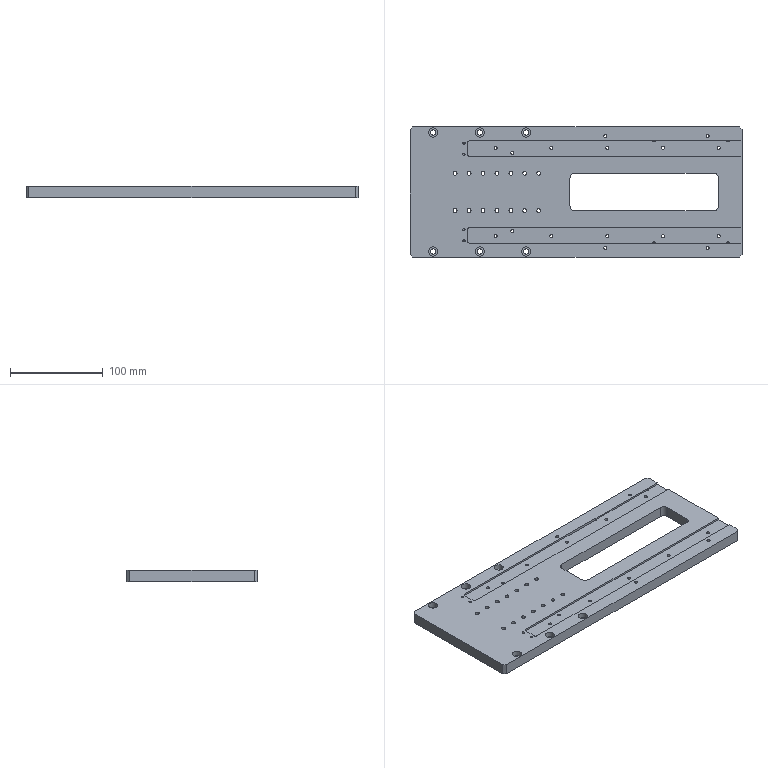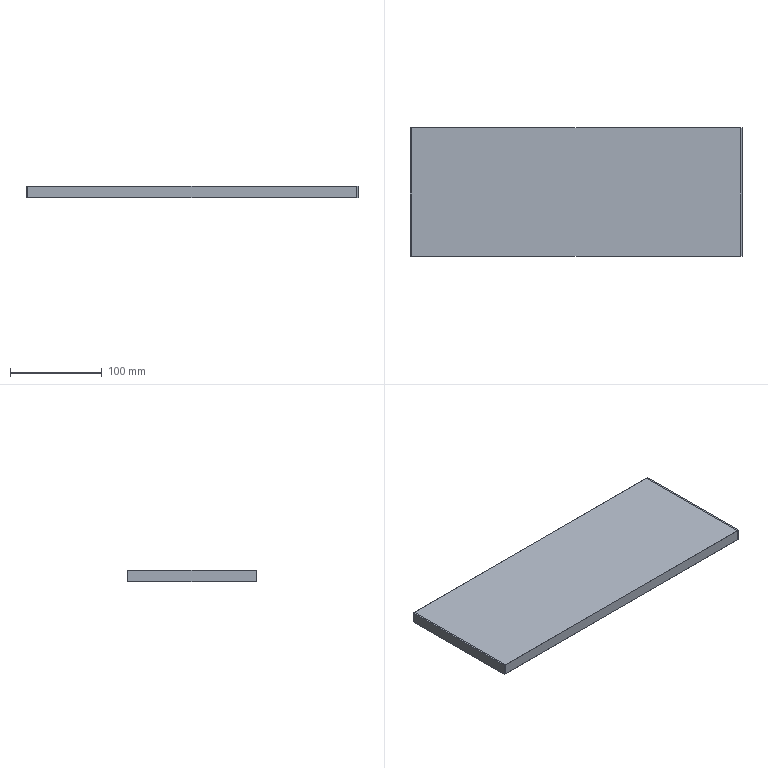CAM job | NX | 3+2 milling, drilling | part box 357 x 140 x 12 mm | stock box 361 x 140 x 12 mm
Tools:
number,name,description,diameter,corner_radius,flute_length,length,flutes
15,D10,Milling Tool-5 Parameters,10.0,0.0,50.0,75.0,2
1,D6A45,Milling Tool-5 Parameters,6.0,0.0,50.0,75.0,2
2,2.5ZT,Drilling Tool,2.0,0.0,35.0,50.0,2
9,5.5ZT,Drilling Tool,5.5,0.0,35.0,50.0,2
4,4.2ZT,Drilling Tool,4.2,0.0,35.0,50.0,2
3,3.3ZT,Drilling Tool,3.3,0.0,35.0,50.0,2
14,D10JING,Milling Tool-5 Parameters,10.0,0.0,50.0,75.0,2
11,D4,Milling Tool-5 Parameters,4.0,0.0,50.0,75.0,2
16,D3,Milling Tool-5 Parameters,3.0,0.0,50.0,75.0,2
Operations:
program,operation,operation_type,tool,method,geometry_group,spindle_rpm,surface_speed,feed_per_tooth,feed_cut,feed_plunge,cut_length_mm,path_length_mm,cut_time_min,machine_time_min
1,DRILLING,Operation,D6A45,METHOD,A,9500.0,179.0,0.0132,250.0,0.0,160.0,1561.72,0.64,0.7802
1,DRILLING_COPY_COPY_COPY,Operation,2.5ZT,METHOD,A,2000.0,12.0,0.025,100.0,0.0,44.403,263.601,0.444,0.466
1,DRILLING_COPY_COPY,Operation,5.5ZT,METHOD,A,2000.0,21.0,0.075,300.0,0.0,102.914,609.223,0.343,0.3937
1,DRILLING_COPY_COPY_COPY_COPY,Operation,4.2ZT,METHOD,A,2000.0,26.0,0.075,300.0,0.0,234.665,792.008,0.7822,0.838
1,DRILLING_COPY_COPY_COPY_1,Operation,3.3ZT,METHOD,A,2026.0,21.0,0.0494,200.0,0.0,197.897,1067.339,0.9895,1.076
1,ZLEVEL_PROFILE,ZLevelMilling,D10,METHOD,A,9500.0,298.0,0.1579,3000.0,1000.0,4052.941,4600.819,1.418,1.472
1,PLANAR_MILL,PlanarMilling,D10,METHOD,A,9500.0,298.0,0.1579,3000.0,1000.0,15174.82,15792.257,5.44,5.502
1,FLOOR_WALL,VolumeBased25DMillingOperation,D10,METHOD,A,9500.0,298.0,0.1316,2500.0,100.0,2448.682,2669.402,0.9795,1.002
1,FLOOR_WALL_1,VolumeBased25DMillingOperation,D10JING,METHOD,A,9500.0,298.0,0.0658,1250.0,100.0,554.732,1418.31,0.4438,0.5301
1,ZLEVEL_PROFILE_COPY,ZLevelMilling,D4,METHOD,A,9500.0,119.0,0.0789,1500.0,1000.0,160.342,566.633,0.1143,0.1549
1,FLOOR_WALL_COPY,VolumeBased25DMillingOperation,D4,METHOD,A,9500.0,298.0,0.0711,1350.0,100.0,5980.881,6212.076,4.43,4.453
1,HOLE_MILLING,CylinderMilling,D4,METHOD,A,9500.0,119.0,0.0789,1500.0,100.0,2837.119,3593.519,1.891,1.967
1,PLANAR_MILL_COPY,PlanarMilling,D6A45,METHOD,A,8500.0,160.0,0.0735,1250.0,100.0,2985.292,5917.419,2.388,2.681
2,DRILLING_COPY,Operation,D6A45,METHOD,B,9500.0,179.0,0.0132,250.0,0.0,16.0,370.554,0.064,0.0995
2,DRILLING_COPY_COPY_1,Operation,2.5ZT,METHOD,B,1500.0,28.0,0.04,120.0,0.0,54.403,447.361,0.4534,0.4927
2,PLANAR_MILL_COPY_COPY,PlanarMilling,D6A45,METHOD,B,8500.0,160.0,0.0735,1250.0,100.0,1830.903,5553.476,1.465,1.837
3,DRILLING_COPY_1,Operation,D6A45,METHOD,C,9500.0,179.0,0.0132,250.0,0.0,16.0,303.229,0.064,0.0927
3,DRILLING_COPY_COPY_COPY_COPY_COPY,Operation,4.2ZT,METHOD,C,2000.0,26.0,0.075,300.0,0.0,33.524,175.147,0.1117,0.1259
3,DRILLING_COPY_COPY_COPY_COPY_COPY_COPY,Operation,4.2ZT,METHOD,C,2000.0,26.0,0.075,300.0,0.0,28.524,239.585,0.0951,0.1162
3,ZLEVEL_PROFILE_1_1,ZLevelMilling,D3,METHOD,C,9500.0,89.0,0.0632,1200.0,1000.0,741.538,994.178,0.6288,0.654
3,PLANAR_MILL_COPY_COPY_COPY,PlanarMilling,D6A45,METHOD,C,8500.0,160.0,0.0735,1250.0,100.0,67.579,423.977,0.0541,0.0897
3,刀补,ZLevelMilling,D3,METHOD,C,9500.0,89.0,0.0632,1200.0,1000.0,93.009,352.347,0.0781,0.1041